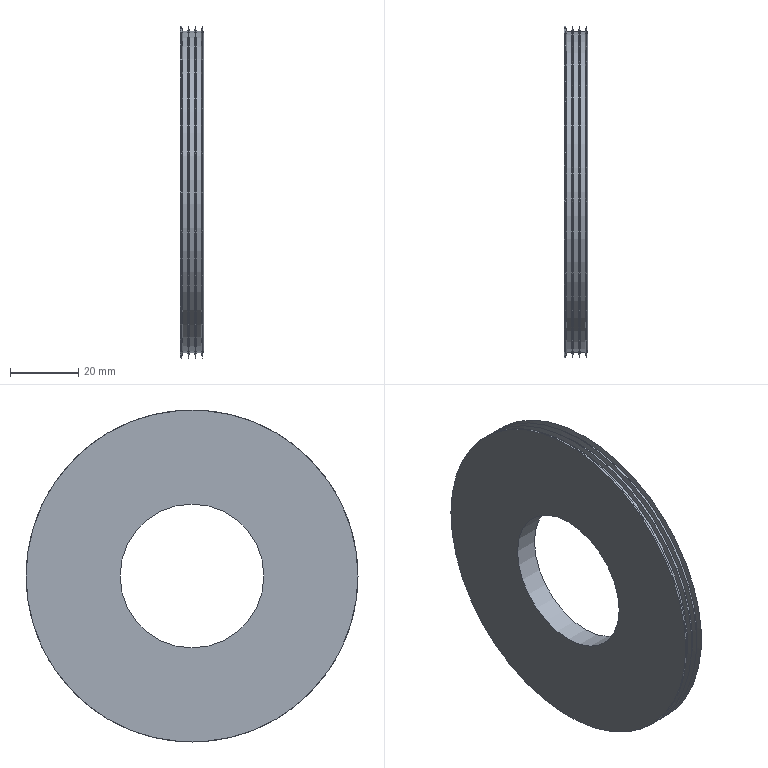Part | NX | features DATUM_CSYS 3, SKETCH 2, CHAMFER 1, EXTRUDE 1, SWP104 1 | 1 solid | 14 faces | box 7 x 97 x 97 mm | volume 39442 mm3 | cone 7 | cylinder 5 | plane 2 | commonest cylinder face diameters 94 x3 42 x1 97 x1
STEP:
#1=CARTESIAN_POINT('',(0.5,0.,-48.5));
#2=VERTEX_POINT('',#1);
#3=CARTESIAN_POINT('',(0.5,0.,0.));
#4=DIRECTION('',(1.,0.,0.));
#5=DIRECTION('',(0.,0.,-1.));
#6=AXIS2_PLACEMENT_3D('',#3,#4,#5);
#7=CIRCLE('',#6,48.5);
#8=EDGE_CURVE('',#2,#2,#7,.F.);
#9=ORIENTED_EDGE('',*,*,#8,.T.);
#10=EDGE_LOOP('',(#9));
#11=FACE_BOUND('',#10,.T.);
#12=CARTESIAN_POINT('',(0.,48.5,0.));
#13=VERTEX_POINT('',#12);
#14=CARTESIAN_POINT('',(0.,0.,0.));
#15=DIRECTION('',(1.,0.,0.));
#16=DIRECTION('',(0.,1.,0.));
#17=AXIS2_PLACEMENT_3D('',#14,#15,#16);
#18=CIRCLE('',#17,48.5);
#19=EDGE_CURVE('',#13,#13,#18,.T.);
#20=ORIENTED_EDGE('',*,*,#19,.T.);
#21=EDGE_LOOP('',(#20));
#22=FACE_BOUND('',#21,.T.);
#23=CARTESIAN_POINT('',(7.,0.,0.));
#24=DIRECTION('',(-1.,0.,0.));
#25=DIRECTION('',(0.,0.,1.));
#26=AXIS2_PLACEMENT_3D('',#23,#24,#25);
#27=CYLINDRICAL_SURFACE('',#26,48.5);
#28=ADVANCED_FACE('',(#11,#22),#27,.T.);
#29=CARTESIAN_POINT('',(7.,21.,0.));
#30=VERTEX_POINT('',#29);
#31=CARTESIAN_POINT('',(7.,0.,0.));
#32=DIRECTION('',(1.,0.,0.));
#33=DIRECTION('',(0.,1.,0.));
#34=AXIS2_PLACEMENT_3D('',#31,#32,#33);
#35=CIRCLE('',#34,21.);
#36=EDGE_CURVE('',#30,#30,#35,.T.);
#37=ORIENTED_EDGE('',*,*,#36,.T.);
#38=EDGE_LOOP('',(#37));
#39=FACE_BOUND('',#38,.T.);
#40=CARTESIAN_POINT('',(0.,21.,0.));
#41=VERTEX_POINT('',#40);
#42=CARTESIAN_POINT('',(0.,0.,0.));
#43=DIRECTION('',(1.,0.,0.));
#44=DIRECTION('',(0.,1.,0.));
#45=AXIS2_PLACEMENT_3D('',#42,#43,#44);
#46=CIRCLE('',#45,21.);
#47=EDGE_CURVE('',#41,#41,#46,.T.);
#48=ORIENTED_EDGE('',*,*,#47,.F.);
#49=EDGE_LOOP('',(#48));
#50=FACE_BOUND('',#49,.T.);
#51=CARTESIAN_POINT('',(7.,0.,0.));
#52=DIRECTION('',(-1.,0.,0.));
#53=DIRECTION('',(0.,0.,1.));
#54=AXIS2_PLACEMENT_3D('',#51,#52,#53);
#55=CYLINDRICAL_SURFACE('',#54,21.);
#56=ADVANCED_FACE('',(#39,#50),#55,.F.);
#57=CARTESIAN_POINT('',(7.,0.,-45.5));
#58=VERTEX_POINT('',#57);
#59=CARTESIAN_POINT('',(7.,0.,0.));
#60=DIRECTION('',(1.,0.,0.));
#61=DIRECTION('',(0.,0.,-1.));
#62=AXIS2_PLACEMENT_3D('',#59,#60,#61);
#63=CIRCLE('',#62,45.5);
#64=EDGE_CURVE('',#58,#58,#63,.T.);
#65=ORIENTED_EDGE('',*,*,#64,.T.);
#66=EDGE_LOOP('',(#65));
#67=FACE_BOUND('',#66,.T.);
#68=ORIENTED_EDGE('',*,*,#36,.F.);
#69=EDGE_LOOP('',(#68));
#70=FACE_BOUND('',#69,.T.);
#71=CARTESIAN_POINT('',(7.,0.,0.));
#72=DIRECTION('',(1.,0.,0.));
#73=DIRECTION('',(0.,0.,-1.));
#74=AXIS2_PLACEMENT_3D('',#71,#72,#73);
#75=PLANE('',#74);
#76=ADVANCED_FACE('',(#67,#70),#75,.T.);
#77=ORIENTED_EDGE('',*,*,#19,.F.);
#78=EDGE_LOOP('',(#77));
#79=FACE_BOUND('',#78,.T.);
#80=ORIENTED_EDGE('',*,*,#47,.T.);
#81=EDGE_LOOP('',(#80));
#82=FACE_BOUND('',#81,.T.);
#83=CARTESIAN_POINT('',(0.,0.,0.));
#84=DIRECTION('',(1.,0.,0.));
#85=DIRECTION('',(0.,0.,-1.));
#86=AXIS2_PLACEMENT_3D('',#83,#84,#85);
#87=PLANE('',#86);
#88=ADVANCED_FACE('',(#79,#82),#87,.F.);
#89=CARTESIAN_POINT('',(4.75,0.,47.));
#90=VERTEX_POINT('',#89);
#91=CARTESIAN_POINT('',(4.75,0.,0.));
#92=DIRECTION('',(-1.,0.,0.));
#93=DIRECTION('',(0.,0.,1.));
#94=AXIS2_PLACEMENT_3D('',#91,#92,#93);
#95=CIRCLE('',#94,47.);
#96=EDGE_CURVE('',#90,#90,#95,.F.);
#97=ORIENTED_EDGE('',*,*,#96,.T.);
#98=EDGE_LOOP('',(#97));
#99=FACE_BOUND('',#98,.T.);
#100=CARTESIAN_POINT('',(6.25,0.,-47.));
#101=VERTEX_POINT('',#100);
#102=CARTESIAN_POINT('',(6.25,0.,0.));
#103=DIRECTION('',(1.,0.,0.));
#104=DIRECTION('',(0.,0.,-1.));
#105=AXIS2_PLACEMENT_3D('',#102,#103,#104);
#106=CIRCLE('',#105,47.);
#107=EDGE_CURVE('',#101,#101,#106,.F.);
#108=ORIENTED_EDGE('',*,*,#107,.T.);
#109=EDGE_LOOP('',(#108));
#110=FACE_BOUND('',#109,.T.);
#111=CARTESIAN_POINT('',(0.,0.,0.));
#112=DIRECTION('',(-1.,0.,0.));
#113=DIRECTION('',(0.,0.,1.));
#114=AXIS2_PLACEMENT_3D('',#111,#112,#113);
#115=CYLINDRICAL_SURFACE('',#114,47.);
#116=ADVANCED_FACE('',(#99,#110),#115,.T.);
#117=CARTESIAN_POINT('',(2.75,0.,47.));
#118=VERTEX_POINT('',#117);
#119=CARTESIAN_POINT('',(2.75,0.,0.));
#120=DIRECTION('',(-1.,0.,0.));
#121=DIRECTION('',(0.,0.,1.));
#122=AXIS2_PLACEMENT_3D('',#119,#120,#121);
#123=CIRCLE('',#122,47.);
#124=EDGE_CURVE('',#118,#118,#123,.F.);
#125=ORIENTED_EDGE('',*,*,#124,.T.);
#126=EDGE_LOOP('',(#125));
#127=FACE_BOUND('',#126,.T.);
#128=CARTESIAN_POINT('',(4.25,0.,-47.));
#129=VERTEX_POINT('',#128);
#130=CARTESIAN_POINT('',(4.25,0.,0.));
#131=DIRECTION('',(1.,0.,0.));
#132=DIRECTION('',(0.,0.,-1.));
#133=AXIS2_PLACEMENT_3D('',#130,#131,#132);
#134=CIRCLE('',#133,47.);
#135=EDGE_CURVE('',#129,#129,#134,.F.);
#136=ORIENTED_EDGE('',*,*,#135,.T.);
#137=EDGE_LOOP('',(#136));
#138=FACE_BOUND('',#137,.T.);
#139=CARTESIAN_POINT('',(0.,0.,0.));
#140=DIRECTION('',(-1.,0.,0.));
#141=DIRECTION('',(0.,0.,1.));
#142=AXIS2_PLACEMENT_3D('',#139,#140,#141);
#143=CYLINDRICAL_SURFACE('',#142,47.);
#144=ADVANCED_FACE('',(#127,#138),#143,.T.);
#145=CARTESIAN_POINT('',(2.25,0.,-47.));
#146=VERTEX_POINT('',#145);
#147=CARTESIAN_POINT('',(2.25,0.,0.));
#148=DIRECTION('',(1.,0.,0.));
#149=DIRECTION('',(0.,0.,-1.));
#150=AXIS2_PLACEMENT_3D('',#147,#148,#149);
#151=CIRCLE('',#150,47.);
#152=EDGE_CURVE('',#146,#146,#151,.F.);
#153=ORIENTED_EDGE('',*,*,#152,.T.);
#154=EDGE_LOOP('',(#153));
#155=FACE_BOUND('',#154,.T.);
#156=CARTESIAN_POINT('',(0.75,0.,47.));
#157=VERTEX_POINT('',#156);
#158=CARTESIAN_POINT('',(0.75,0.,0.));
#159=DIRECTION('',(-1.,0.,0.));
#160=DIRECTION('',(0.,0.,1.));
#161=AXIS2_PLACEMENT_3D('',#158,#159,#160);
#162=CIRCLE('',#161,47.);
#163=EDGE_CURVE('',#157,#157,#162,.F.);
#164=ORIENTED_EDGE('',*,*,#163,.T.);
#165=EDGE_LOOP('',(#164));
#166=FACE_BOUND('',#165,.T.);
#167=CARTESIAN_POINT('',(0.,0.,0.));
#168=DIRECTION('',(-1.,0.,0.));
#169=DIRECTION('',(0.,0.,1.));
#170=AXIS2_PLACEMENT_3D('',#167,#168,#169);
#171=CYLINDRICAL_SURFACE('',#170,47.);
#172=ADVANCED_FACE('',(#155,#166),#171,.T.);
#173=ORIENTED_EDGE('',*,*,#107,.F.);
#174=EDGE_LOOP('',(#173));
#175=FACE_BOUND('',#174,.T.);
#176=CARTESIAN_POINT('',(6.5,0.,48.5));
#177=VERTEX_POINT('',#176);
#178=CARTESIAN_POINT('',(6.5,0.,0.));
#179=DIRECTION('',(-1.,0.,0.));
#180=DIRECTION('',(0.,0.,1.));
#181=AXIS2_PLACEMENT_3D('',#178,#179,#180);
#182=CIRCLE('',#181,48.5);
#183=EDGE_CURVE('',#177,#177,#182,.F.);
#184=ORIENTED_EDGE('',*,*,#183,.F.);
#185=EDGE_LOOP('',(#184));
#186=FACE_BOUND('',#185,.T.);
#187=CARTESIAN_POINT('',(6.,0.,0.));
#188=DIRECTION('',(1.,0.,0.));
#189=DIRECTION('',(0.,0.,-1.));
#190=AXIS2_PLACEMENT_3D('',#187,#188,#189);
#191=CONICAL_SURFACE('',#190,45.5,1.406);
#192=ADVANCED_FACE('',(#175,#186),#191,.T.);
#193=ORIENTED_EDGE('',*,*,#183,.T.);
#194=EDGE_LOOP('',(#193));
#195=FACE_BOUND('',#194,.T.);
#196=ORIENTED_EDGE('',*,*,#64,.F.);
#197=EDGE_LOOP('',(#196));
#198=FACE_BOUND('',#197,.T.);
#199=CARTESIAN_POINT('',(7.,0.,0.));
#200=DIRECTION('',(-1.,0.,0.));
#201=DIRECTION('',(0.,0.,1.));
#202=AXIS2_PLACEMENT_3D('',#199,#200,#201);
#203=CONICAL_SURFACE('',#202,45.5,1.406);
#204=ADVANCED_FACE('',(#195,#198),#203,.T.);
#205=ORIENTED_EDGE('',*,*,#135,.F.);
#206=EDGE_LOOP('',(#205));
#207=FACE_BOUND('',#206,.T.);
#208=CARTESIAN_POINT('',(4.5,0.,48.5));
#209=VERTEX_POINT('',#208);
#210=CARTESIAN_POINT('',(4.5,0.,0.));
#211=DIRECTION('',(-1.,0.,0.));
#212=DIRECTION('',(0.,0.,1.));
#213=AXIS2_PLACEMENT_3D('',#210,#211,#212);
#214=CIRCLE('',#213,48.5);
#215=EDGE_CURVE('',#209,#209,#214,.F.);
#216=ORIENTED_EDGE('',*,*,#215,.F.);
#217=EDGE_LOOP('',(#216));
#218=FACE_BOUND('',#217,.T.);
#219=CARTESIAN_POINT('',(4.,0.,0.));
#220=DIRECTION('',(1.,0.,0.));
#221=DIRECTION('',(0.,0.,-1.));
#222=AXIS2_PLACEMENT_3D('',#219,#220,#221);
#223=CONICAL_SURFACE('',#222,45.5,1.406);
#224=ADVANCED_FACE('',(#207,#218),#223,.T.);
#225=ORIENTED_EDGE('',*,*,#215,.T.);
#226=EDGE_LOOP('',(#225));
#227=FACE_BOUND('',#226,.T.);
#228=ORIENTED_EDGE('',*,*,#96,.F.);
#229=EDGE_LOOP('',(#228));
#230=FACE_BOUND('',#229,.T.);
#231=CARTESIAN_POINT('',(5.,0.,0.));
#232=DIRECTION('',(-1.,0.,0.));
#233=DIRECTION('',(0.,0.,1.));
#234=AXIS2_PLACEMENT_3D('',#231,#232,#233);
#235=CONICAL_SURFACE('',#234,45.5,1.406);
#236=ADVANCED_FACE('',(#227,#230),#235,.T.);
#237=ORIENTED_EDGE('',*,*,#8,.F.);
#238=EDGE_LOOP('',(#237));
#239=FACE_BOUND('',#238,.T.);
#240=ORIENTED_EDGE('',*,*,#163,.F.);
#241=EDGE_LOOP('',(#240));
#242=FACE_BOUND('',#241,.T.);
#243=CARTESIAN_POINT('',(1.,0.,0.));
#244=DIRECTION('',(-1.,0.,0.));
#245=DIRECTION('',(0.,0.,1.));
#246=AXIS2_PLACEMENT_3D('',#243,#244,#245);
#247=CONICAL_SURFACE('',#246,45.5,1.406);
#248=ADVANCED_FACE('',(#239,#242),#247,.T.);
#249=ORIENTED_EDGE('',*,*,#124,.F.);
#250=EDGE_LOOP('',(#249));
#251=FACE_BOUND('',#250,.T.);
#252=CARTESIAN_POINT('',(2.5,0.,-48.5));
#253=VERTEX_POINT('',#252);
#254=CARTESIAN_POINT('',(2.5,0.,0.));
#255=DIRECTION('',(1.,0.,0.));
#256=DIRECTION('',(0.,0.,-1.));
#257=AXIS2_PLACEMENT_3D('',#254,#255,#256);
#258=CIRCLE('',#257,48.5);
#259=EDGE_CURVE('',#253,#253,#258,.F.);
#260=ORIENTED_EDGE('',*,*,#259,.F.);
#261=EDGE_LOOP('',(#260));
#262=FACE_BOUND('',#261,.T.);
#263=CARTESIAN_POINT('',(3.,0.,0.));
#264=DIRECTION('',(-1.,0.,0.));
#265=DIRECTION('',(0.,0.,1.));
#266=AXIS2_PLACEMENT_3D('',#263,#264,#265);
#267=CONICAL_SURFACE('',#266,45.5,1.406);
#268=ADVANCED_FACE('',(#251,#262),#267,.T.);
#269=ORIENTED_EDGE('',*,*,#259,.T.);
#270=EDGE_LOOP('',(#269));
#271=FACE_BOUND('',#270,.T.);
#272=ORIENTED_EDGE('',*,*,#152,.F.);
#273=EDGE_LOOP('',(#272));
#274=FACE_BOUND('',#273,.T.);
#275=CARTESIAN_POINT('',(2.,0.,0.));
#276=DIRECTION('',(1.,0.,0.));
#277=DIRECTION('',(0.,0.,-1.));
#278=AXIS2_PLACEMENT_3D('',#275,#276,#277);
#279=CONICAL_SURFACE('',#278,45.5,1.406);
#280=ADVANCED_FACE('',(#271,#274),#279,.T.);
#281=CLOSED_SHELL('',(#28,#56,#76,#88,#116,#144,#172,#192,#204,#224,#236,#248,#268,#280));
#282=MANIFOLD_SOLID_BREP('',#281);
#283=(LENGTH_UNIT()NAMED_UNIT(*)SI_UNIT(.MILLI.,.METRE.));
#284=UNCERTAINTY_MEASURE_WITH_UNIT(LENGTH_MEASURE(0.00001),#283,'','');
#285=(NAMED_UNIT(*)PLANE_ANGLE_UNIT()SI_UNIT($,.RADIAN.));
#286=(NAMED_UNIT(*)SI_UNIT($,.STERADIAN.)SOLID_ANGLE_UNIT());
#287=(GEOMETRIC_REPRESENTATION_CONTEXT(3)GLOBAL_UNCERTAINTY_ASSIGNED_CONTEXT((#284))GLOBAL_UNIT_ASSIGNED_CONTEXT((#283,#285,#286))REPRESENTATION_CONTEXT('',''));
#288=ADVANCED_BREP_SHAPE_REPRESENTATION('',(#282),#287);